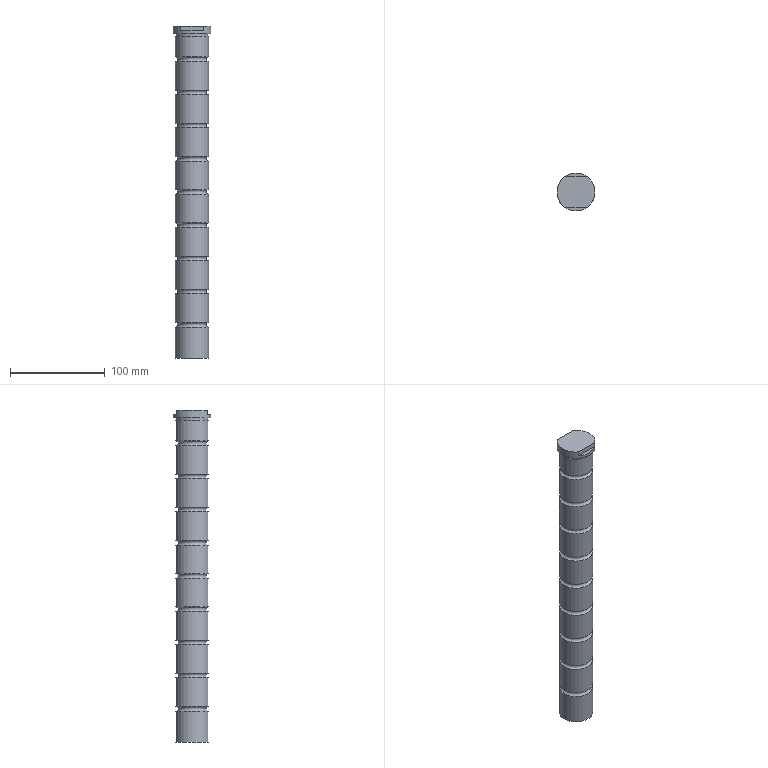Part | STEP file | 1_id442_xmt_txt | 1 solid | 33 faces | box 40 x 40 x 350 mm | volume 322067 mm3 | cylinder 14 | torus 9 | plane 8 | cone 2 | commonest cylinder face diameters 35 x10 13.6 x1 16 x1 33 x1 40 x1
STEP:
#1=CARTESIAN_POINT('',(144.5,302.,-131.5));
#2=VERTEX_POINT('',#1);
#3=CARTESIAN_POINT('',(162.,302.,-131.5));
#4=DIRECTION('',(0.,0.,-1.));
#5=DIRECTION('',(-1.,0.,0.));
#6=AXIS2_PLACEMENT_3D('',#3,#4,#5);
#7=CIRCLE('',#6,17.5);
#8=EDGE_CURVE('',#2,#2,#7,.T.);
#9=ORIENTED_EDGE('',*,*,#8,.F.);
#10=EDGE_LOOP('',(#9));
#11=FACE_BOUND('',#10,.T.);
#12=CARTESIAN_POINT('',(144.5,302.,-126.5));
#13=VERTEX_POINT('',#12);
#14=CARTESIAN_POINT('',(162.,302.,-126.5));
#15=DIRECTION('',(0.,0.,1.));
#16=DIRECTION('',(-1.,0.,0.));
#17=AXIS2_PLACEMENT_3D('',#14,#15,#16);
#18=CIRCLE('',#17,17.5);
#19=EDGE_CURVE('',#13,#13,#18,.T.);
#20=ORIENTED_EDGE('',*,*,#19,.F.);
#21=EDGE_LOOP('',(#20));
#22=FACE_BOUND('',#21,.T.);
#23=CARTESIAN_POINT('',(162.,302.,-129.));
#24=DIRECTION('',(0.,0.,-1.));
#25=DIRECTION('',(1.,0.,0.));
#26=AXIS2_PLACEMENT_3D('',#23,#24,#25);
#27=TOROIDAL_SURFACE('',#26,17.5,2.5);
#28=ADVANCED_FACE('',(#11,#22),#27,.F.);
#29=CARTESIAN_POINT('',(144.5,302.,-96.5));
#30=VERTEX_POINT('',#29);
#31=CARTESIAN_POINT('',(162.,302.,-96.5));
#32=DIRECTION('',(0.,0.,-1.));
#33=DIRECTION('',(-1.,0.,0.));
#34=AXIS2_PLACEMENT_3D('',#31,#32,#33);
#35=CIRCLE('',#34,17.5);
#36=EDGE_CURVE('',#30,#30,#35,.T.);
#37=ORIENTED_EDGE('',*,*,#36,.F.);
#38=EDGE_LOOP('',(#37));
#39=FACE_BOUND('',#38,.T.);
#40=CARTESIAN_POINT('',(144.5,302.,-91.5));
#41=VERTEX_POINT('',#40);
#42=CARTESIAN_POINT('',(162.,302.,-91.5));
#43=DIRECTION('',(0.,0.,1.));
#44=DIRECTION('',(-1.,0.,0.));
#45=AXIS2_PLACEMENT_3D('',#42,#43,#44);
#46=CIRCLE('',#45,17.5);
#47=EDGE_CURVE('',#41,#41,#46,.T.);
#48=ORIENTED_EDGE('',*,*,#47,.F.);
#49=EDGE_LOOP('',(#48));
#50=FACE_BOUND('',#49,.T.);
#51=CARTESIAN_POINT('',(162.,302.,-94.));
#52=DIRECTION('',(0.,0.,-1.));
#53=DIRECTION('',(1.,0.,0.));
#54=AXIS2_PLACEMENT_3D('',#51,#52,#53);
#55=TOROIDAL_SURFACE('',#54,17.5,2.5);
#56=ADVANCED_FACE('',(#39,#50),#55,.F.);
#57=CARTESIAN_POINT('',(144.5,302.,-61.5));
#58=VERTEX_POINT('',#57);
#59=CARTESIAN_POINT('',(162.,302.,-61.5));
#60=DIRECTION('',(0.,0.,-1.));
#61=DIRECTION('',(-1.,0.,0.));
#62=AXIS2_PLACEMENT_3D('',#59,#60,#61);
#63=CIRCLE('',#62,17.5);
#64=EDGE_CURVE('',#58,#58,#63,.T.);
#65=ORIENTED_EDGE('',*,*,#64,.F.);
#66=EDGE_LOOP('',(#65));
#67=FACE_BOUND('',#66,.T.);
#68=CARTESIAN_POINT('',(144.5,302.,-56.5));
#69=VERTEX_POINT('',#68);
#70=CARTESIAN_POINT('',(162.,302.,-56.5));
#71=DIRECTION('',(0.,0.,1.));
#72=DIRECTION('',(-1.,0.,0.));
#73=AXIS2_PLACEMENT_3D('',#70,#71,#72);
#74=CIRCLE('',#73,17.5);
#75=EDGE_CURVE('',#69,#69,#74,.T.);
#76=ORIENTED_EDGE('',*,*,#75,.F.);
#77=EDGE_LOOP('',(#76));
#78=FACE_BOUND('',#77,.T.);
#79=CARTESIAN_POINT('',(162.,302.,-59.));
#80=DIRECTION('',(0.,0.,-1.));
#81=DIRECTION('',(1.,0.,0.));
#82=AXIS2_PLACEMENT_3D('',#79,#80,#81);
#83=TOROIDAL_SURFACE('',#82,17.5,2.5);
#84=ADVANCED_FACE('',(#67,#78),#83,.F.);
#85=CARTESIAN_POINT('',(144.5,302.,-26.5));
#86=VERTEX_POINT('',#85);
#87=CARTESIAN_POINT('',(162.,302.,-26.5));
#88=DIRECTION('',(0.,0.,-1.));
#89=DIRECTION('',(-1.,0.,0.));
#90=AXIS2_PLACEMENT_3D('',#87,#88,#89);
#91=CIRCLE('',#90,17.5);
#92=EDGE_CURVE('',#86,#86,#91,.T.);
#93=ORIENTED_EDGE('',*,*,#92,.F.);
#94=EDGE_LOOP('',(#93));
#95=FACE_BOUND('',#94,.T.);
#96=CARTESIAN_POINT('',(144.5,302.,-21.5));
#97=VERTEX_POINT('',#96);
#98=CARTESIAN_POINT('',(162.,302.,-21.5));
#99=DIRECTION('',(0.,0.,1.));
#100=DIRECTION('',(-1.,0.,0.));
#101=AXIS2_PLACEMENT_3D('',#98,#99,#100);
#102=CIRCLE('',#101,17.5);
#103=EDGE_CURVE('',#97,#97,#102,.T.);
#104=ORIENTED_EDGE('',*,*,#103,.F.);
#105=EDGE_LOOP('',(#104));
#106=FACE_BOUND('',#105,.T.);
#107=CARTESIAN_POINT('',(162.,302.,-24.));
#108=DIRECTION('',(0.,0.,-1.));
#109=DIRECTION('',(1.,0.,0.));
#110=AXIS2_PLACEMENT_3D('',#107,#108,#109);
#111=TOROIDAL_SURFACE('',#110,17.5,2.5);
#112=ADVANCED_FACE('',(#95,#106),#111,.F.);
#113=CARTESIAN_POINT('',(144.5,302.,8.5));
#114=VERTEX_POINT('',#113);
#115=CARTESIAN_POINT('',(162.,302.,8.5));
#116=DIRECTION('',(0.,0.,-1.));
#117=DIRECTION('',(-1.,0.,0.));
#118=AXIS2_PLACEMENT_3D('',#115,#116,#117);
#119=CIRCLE('',#118,17.5);
#120=EDGE_CURVE('',#114,#114,#119,.T.);
#121=ORIENTED_EDGE('',*,*,#120,.F.);
#122=EDGE_LOOP('',(#121));
#123=FACE_BOUND('',#122,.T.);
#124=CARTESIAN_POINT('',(144.5,302.,13.5));
#125=VERTEX_POINT('',#124);
#126=CARTESIAN_POINT('',(162.,302.,13.5));
#127=DIRECTION('',(0.,0.,1.));
#128=DIRECTION('',(-1.,0.,0.));
#129=AXIS2_PLACEMENT_3D('',#126,#127,#128);
#130=CIRCLE('',#129,17.5);
#131=EDGE_CURVE('',#125,#125,#130,.T.);
#132=ORIENTED_EDGE('',*,*,#131,.F.);
#133=EDGE_LOOP('',(#132));
#134=FACE_BOUND('',#133,.T.);
#135=CARTESIAN_POINT('',(162.,302.,11.));
#136=DIRECTION('',(0.,0.,-1.));
#137=DIRECTION('',(1.,0.,0.));
#138=AXIS2_PLACEMENT_3D('',#135,#136,#137);
#139=TOROIDAL_SURFACE('',#138,17.5,2.5);
#140=ADVANCED_FACE('',(#123,#134),#139,.F.);
#141=CARTESIAN_POINT('',(144.5,302.,43.5));
#142=VERTEX_POINT('',#141);
#143=CARTESIAN_POINT('',(162.,302.,43.5));
#144=DIRECTION('',(0.,0.,-1.));
#145=DIRECTION('',(-1.,0.,0.));
#146=AXIS2_PLACEMENT_3D('',#143,#144,#145);
#147=CIRCLE('',#146,17.5);
#148=EDGE_CURVE('',#142,#142,#147,.T.);
#149=ORIENTED_EDGE('',*,*,#148,.F.);
#150=EDGE_LOOP('',(#149));
#151=FACE_BOUND('',#150,.T.);
#152=CARTESIAN_POINT('',(144.5,302.,48.5));
#153=VERTEX_POINT('',#152);
#154=CARTESIAN_POINT('',(162.,302.,48.5));
#155=DIRECTION('',(0.,0.,1.));
#156=DIRECTION('',(-1.,0.,0.));
#157=AXIS2_PLACEMENT_3D('',#154,#155,#156);
#158=CIRCLE('',#157,17.5);
#159=EDGE_CURVE('',#153,#153,#158,.T.);
#160=ORIENTED_EDGE('',*,*,#159,.F.);
#161=EDGE_LOOP('',(#160));
#162=FACE_BOUND('',#161,.T.);
#163=CARTESIAN_POINT('',(162.,302.,46.));
#164=DIRECTION('',(0.,0.,-1.));
#165=DIRECTION('',(1.,0.,0.));
#166=AXIS2_PLACEMENT_3D('',#163,#164,#165);
#167=TOROIDAL_SURFACE('',#166,17.5,2.5);
#168=ADVANCED_FACE('',(#151,#162),#167,.F.);
#169=CARTESIAN_POINT('',(144.5,302.,78.5));
#170=VERTEX_POINT('',#169);
#171=CARTESIAN_POINT('',(162.,302.,78.5));
#172=DIRECTION('',(0.,0.,-1.));
#173=DIRECTION('',(-1.,0.,0.));
#174=AXIS2_PLACEMENT_3D('',#171,#172,#173);
#175=CIRCLE('',#174,17.5);
#176=EDGE_CURVE('',#170,#170,#175,.T.);
#177=ORIENTED_EDGE('',*,*,#176,.F.);
#178=EDGE_LOOP('',(#177));
#179=FACE_BOUND('',#178,.T.);
#180=CARTESIAN_POINT('',(144.5,302.,83.5));
#181=VERTEX_POINT('',#180);
#182=CARTESIAN_POINT('',(162.,302.,83.5));
#183=DIRECTION('',(0.,0.,1.));
#184=DIRECTION('',(-1.,0.,0.));
#185=AXIS2_PLACEMENT_3D('',#182,#183,#184);
#186=CIRCLE('',#185,17.5);
#187=EDGE_CURVE('',#181,#181,#186,.T.);
#188=ORIENTED_EDGE('',*,*,#187,.F.);
#189=EDGE_LOOP('',(#188));
#190=FACE_BOUND('',#189,.T.);
#191=CARTESIAN_POINT('',(162.,302.,81.));
#192=DIRECTION('',(0.,0.,-1.));
#193=DIRECTION('',(1.,0.,0.));
#194=AXIS2_PLACEMENT_3D('',#191,#192,#193);
#195=TOROIDAL_SURFACE('',#194,17.5,2.5);
#196=ADVANCED_FACE('',(#179,#190),#195,.F.);
#197=CARTESIAN_POINT('',(144.5,302.,113.5));
#198=VERTEX_POINT('',#197);
#199=CARTESIAN_POINT('',(162.,302.,113.5));
#200=DIRECTION('',(0.,0.,-1.));
#201=DIRECTION('',(-1.,0.,0.));
#202=AXIS2_PLACEMENT_3D('',#199,#200,#201);
#203=CIRCLE('',#202,17.5);
#204=EDGE_CURVE('',#198,#198,#203,.T.);
#205=ORIENTED_EDGE('',*,*,#204,.F.);
#206=EDGE_LOOP('',(#205));
#207=FACE_BOUND('',#206,.T.);
#208=CARTESIAN_POINT('',(144.5,302.,118.5));
#209=VERTEX_POINT('',#208);
#210=CARTESIAN_POINT('',(162.,302.,118.5));
#211=DIRECTION('',(0.,0.,1.));
#212=DIRECTION('',(-1.,0.,0.));
#213=AXIS2_PLACEMENT_3D('',#210,#211,#212);
#214=CIRCLE('',#213,17.5);
#215=EDGE_CURVE('',#209,#209,#214,.T.);
#216=ORIENTED_EDGE('',*,*,#215,.F.);
#217=EDGE_LOOP('',(#216));
#218=FACE_BOUND('',#217,.T.);
#219=CARTESIAN_POINT('',(162.,302.,116.));
#220=DIRECTION('',(0.,0.,-1.));
#221=DIRECTION('',(1.,0.,0.));
#222=AXIS2_PLACEMENT_3D('',#219,#220,#221);
#223=TOROIDAL_SURFACE('',#222,17.5,2.5);
#224=ADVANCED_FACE('',(#207,#218),#223,.F.);
#225=CARTESIAN_POINT('',(144.5,302.,148.5));
#226=VERTEX_POINT('',#225);
#227=CARTESIAN_POINT('',(162.,302.,148.5));
#228=DIRECTION('',(0.,0.,-1.));
#229=DIRECTION('',(-1.,0.,0.));
#230=AXIS2_PLACEMENT_3D('',#227,#228,#229);
#231=CIRCLE('',#230,17.5);
#232=EDGE_CURVE('',#226,#226,#231,.T.);
#233=ORIENTED_EDGE('',*,*,#232,.F.);
#234=EDGE_LOOP('',(#233));
#235=FACE_BOUND('',#234,.T.);
#236=CARTESIAN_POINT('',(144.5,302.,153.5));
#237=VERTEX_POINT('',#236);
#238=CARTESIAN_POINT('',(162.,302.,153.5));
#239=DIRECTION('',(0.,0.,1.));
#240=DIRECTION('',(-1.,0.,0.));
#241=AXIS2_PLACEMENT_3D('',#238,#239,#240);
#242=CIRCLE('',#241,17.5);
#243=EDGE_CURVE('',#237,#237,#242,.T.);
#244=ORIENTED_EDGE('',*,*,#243,.F.);
#245=EDGE_LOOP('',(#244));
#246=FACE_BOUND('',#245,.T.);
#247=CARTESIAN_POINT('',(162.,302.,151.));
#248=DIRECTION('',(0.,0.,-1.));
#249=DIRECTION('',(1.,0.,0.));
#250=AXIS2_PLACEMENT_3D('',#247,#248,#249);
#251=TOROIDAL_SURFACE('',#250,17.5,2.5);
#252=ADVANCED_FACE('',(#235,#246),#251,.F.);
#253=ORIENTED_EDGE('',*,*,#8,.T.);
#254=EDGE_LOOP('',(#253));
#255=FACE_BOUND('',#254,.T.);
#256=CARTESIAN_POINT('',(144.5,302.,-164.));
#257=VERTEX_POINT('',#256);
#258=CARTESIAN_POINT('',(162.,302.,-164.));
#259=DIRECTION('',(0.,0.,-1.));
#260=DIRECTION('',(-1.,0.,0.));
#261=AXIS2_PLACEMENT_3D('',#258,#259,#260);
#262=CIRCLE('',#261,17.5);
#263=EDGE_CURVE('',#257,#257,#262,.T.);
#264=ORIENTED_EDGE('',*,*,#263,.F.);
#265=EDGE_LOOP('',(#264));
#266=FACE_BOUND('',#265,.T.);
#267=CARTESIAN_POINT('',(162.,302.,7.));
#268=DIRECTION('',(0.,0.,-1.));
#269=DIRECTION('',(1.,0.,0.));
#270=AXIS2_PLACEMENT_3D('',#267,#268,#269);
#271=CYLINDRICAL_SURFACE('',#270,17.5);
#272=ADVANCED_FACE('',(#255,#266),#271,.T.);
#273=CARTESIAN_POINT('',(178.5,302.,175.));
#274=VERTEX_POINT('',#273);
#275=CARTESIAN_POINT('',(162.,302.,175.));
#276=DIRECTION('',(0.,0.,-1.));
#277=DIRECTION('',(1.,0.,0.));
#278=AXIS2_PLACEMENT_3D('',#275,#276,#277);
#279=CIRCLE('',#278,16.5);
#280=EDGE_CURVE('',#274,#274,#279,.T.);
#281=ORIENTED_EDGE('',*,*,#280,.F.);
#282=EDGE_LOOP('',(#281));
#283=FACE_BOUND('',#282,.T.);
#284=CARTESIAN_POINT('',(178.5,302.,178.));
#285=VERTEX_POINT('',#284);
#286=CARTESIAN_POINT('',(162.,302.,178.));
#287=DIRECTION('',(0.,0.,1.));
#288=DIRECTION('',(1.,0.,0.));
#289=AXIS2_PLACEMENT_3D('',#286,#287,#288);
#290=CIRCLE('',#289,16.5);
#291=EDGE_CURVE('',#285,#285,#290,.T.);
#292=ORIENTED_EDGE('',*,*,#291,.F.);
#293=EDGE_LOOP('',(#292));
#294=FACE_BOUND('',#293,.T.);
#295=CARTESIAN_POINT('',(162.,302.,176.5));
#296=DIRECTION('',(0.,0.,-1.));
#297=DIRECTION('',(-1.,0.,0.));
#298=AXIS2_PLACEMENT_3D('',#295,#296,#297);
#299=CYLINDRICAL_SURFACE('',#298,16.5);
#300=ADVANCED_FACE('',(#283,#294),#299,.T.);
#301=CARTESIAN_POINT('',(174.,286.,186.));
#302=VERTEX_POINT('',#301);
#303=CARTESIAN_POINT('',(174.,318.,186.));
#304=VERTEX_POINT('',#303);
#305=CARTESIAN_POINT('',(162.,302.,186.));
#306=DIRECTION('',(0.,0.,1.));
#307=DIRECTION('',(-1.,0.,0.));
#308=AXIS2_PLACEMENT_3D('',#305,#306,#307);
#309=CIRCLE('',#308,20.);
#310=EDGE_CURVE('',#302,#304,#309,.T.);
#311=ORIENTED_EDGE('',*,*,#310,.F.);
#312=CARTESIAN_POINT('',(174.,286.,181.));
#313=VERTEX_POINT('',#312);
#314=CARTESIAN_POINT('',(174.,286.,183.5));
#315=DIRECTION('',(0.,0.,-1.));
#316=VECTOR('',#315,1.);
#317=LINE('',#314,#316);
#318=EDGE_CURVE('',#302,#313,#317,.T.);
#319=ORIENTED_EDGE('',*,*,#318,.T.);
#320=CARTESIAN_POINT('',(150.,286.,181.));
#321=VERTEX_POINT('',#320);
#322=CARTESIAN_POINT('',(162.,302.,181.));
#323=DIRECTION('',(0.,0.,-1.));
#324=DIRECTION('',(-1.,0.,0.));
#325=AXIS2_PLACEMENT_3D('',#322,#323,#324);
#326=CIRCLE('',#325,20.);
#327=EDGE_CURVE('',#313,#321,#326,.T.);
#328=ORIENTED_EDGE('',*,*,#327,.T.);
#329=CARTESIAN_POINT('',(150.,286.,186.));
#330=VERTEX_POINT('',#329);
#331=CARTESIAN_POINT('',(150.,286.,183.5));
#332=DIRECTION('',(0.,0.,1.));
#333=VECTOR('',#332,1.);
#334=LINE('',#331,#333);
#335=EDGE_CURVE('',#321,#330,#334,.T.);
#336=ORIENTED_EDGE('',*,*,#335,.T.);
#337=CARTESIAN_POINT('',(150.,318.,186.));
#338=VERTEX_POINT('',#337);
#339=CARTESIAN_POINT('',(162.,302.,186.));
#340=DIRECTION('',(0.,0.,1.));
#341=DIRECTION('',(-1.,0.,0.));
#342=AXIS2_PLACEMENT_3D('',#339,#340,#341);
#343=CIRCLE('',#342,20.);
#344=EDGE_CURVE('',#338,#330,#343,.T.);
#345=ORIENTED_EDGE('',*,*,#344,.F.);
#346=CARTESIAN_POINT('',(150.,318.,181.));
#347=VERTEX_POINT('',#346);
#348=CARTESIAN_POINT('',(150.,318.,183.5));
#349=DIRECTION('',(0.,0.,-1.));
#350=VECTOR('',#349,1.);
#351=LINE('',#348,#350);
#352=EDGE_CURVE('',#338,#347,#351,.T.);
#353=ORIENTED_EDGE('',*,*,#352,.T.);
#354=CARTESIAN_POINT('',(174.,318.,181.));
#355=VERTEX_POINT('',#354);
#356=CARTESIAN_POINT('',(162.,302.,181.));
#357=DIRECTION('',(0.,0.,-1.));
#358=DIRECTION('',(-1.,0.,0.));
#359=AXIS2_PLACEMENT_3D('',#356,#357,#358);
#360=CIRCLE('',#359,20.);
#361=EDGE_CURVE('',#347,#355,#360,.T.);
#362=ORIENTED_EDGE('',*,*,#361,.T.);
#363=CARTESIAN_POINT('',(174.,318.,183.5));
#364=DIRECTION('',(0.,0.,1.));
#365=VECTOR('',#364,1.);
#366=LINE('',#363,#365);
#367=EDGE_CURVE('',#355,#304,#366,.T.);
#368=ORIENTED_EDGE('',*,*,#367,.T.);
#369=EDGE_LOOP('',(#311,#319,#328,#336,#345,#353,#362,#368));
#370=FACE_BOUND('',#369,.T.);
#371=CARTESIAN_POINT('',(142.,302.,178.));
#372=VERTEX_POINT('',#371);
#373=CARTESIAN_POINT('',(162.,302.,178.));
#374=DIRECTION('',(0.,0.,-1.));
#375=DIRECTION('',(-1.,0.,0.));
#376=AXIS2_PLACEMENT_3D('',#373,#374,#375);
#377=CIRCLE('',#376,20.);
#378=EDGE_CURVE('',#372,#372,#377,.T.);
#379=ORIENTED_EDGE('',*,*,#378,.F.);
#380=EDGE_LOOP('',(#379));
#381=FACE_BOUND('',#380,.T.);
#382=CARTESIAN_POINT('',(162.,302.,182.));
#383=DIRECTION('',(0.,0.,-1.));
#384=DIRECTION('',(1.,0.,0.));
#385=AXIS2_PLACEMENT_3D('',#382,#383,#384);
#386=CYLINDRICAL_SURFACE('',#385,20.);
#387=ADVANCED_FACE('',(#370,#381),#386,.T.);
#388=ORIENTED_EDGE('',*,*,#36,.T.);
#389=EDGE_LOOP('',(#388));
#390=FACE_BOUND('',#389,.T.);
#391=ORIENTED_EDGE('',*,*,#19,.T.);
#392=EDGE_LOOP('',(#391));
#393=FACE_BOUND('',#392,.T.);
#394=CARTESIAN_POINT('',(162.,302.,7.));
#395=DIRECTION('',(0.,0.,-1.));
#396=DIRECTION('',(1.,0.,0.));
#397=AXIS2_PLACEMENT_3D('',#394,#395,#396);
#398=CYLINDRICAL_SURFACE('',#397,17.5);
#399=ADVANCED_FACE('',(#390,#393),#398,.T.);
#400=ORIENTED_EDGE('',*,*,#64,.T.);
#401=EDGE_LOOP('',(#400));
#402=FACE_BOUND('',#401,.T.);
#403=ORIENTED_EDGE('',*,*,#47,.T.);
#404=EDGE_LOOP('',(#403));
#405=FACE_BOUND('',#404,.T.);
#406=CARTESIAN_POINT('',(162.,302.,7.));
#407=DIRECTION('',(0.,0.,-1.));
#408=DIRECTION('',(1.,0.,0.));
#409=AXIS2_PLACEMENT_3D('',#406,#407,#408);
#410=CYLINDRICAL_SURFACE('',#409,17.5);
#411=ADVANCED_FACE('',(#402,#405),#410,.T.);
#412=ORIENTED_EDGE('',*,*,#92,.T.);
#413=EDGE_LOOP('',(#412));
#414=FACE_BOUND('',#413,.T.);
#415=ORIENTED_EDGE('',*,*,#75,.T.);
#416=EDGE_LOOP('',(#415));
#417=FACE_BOUND('',#416,.T.);
#418=CARTESIAN_POINT('',(162.,302.,7.));
#419=DIRECTION('',(0.,0.,-1.));
#420=DIRECTION('',(1.,0.,0.));
#421=AXIS2_PLACEMENT_3D('',#418,#419,#420);
#422=CYLINDRICAL_SURFACE('',#421,17.5);
#423=ADVANCED_FACE('',(#414,#417),#422,.T.);
#424=ORIENTED_EDGE('',*,*,#120,.T.);
#425=EDGE_LOOP('',(#424));
#426=FACE_BOUND('',#425,.T.);
#427=ORIENTED_EDGE('',*,*,#103,.T.);
#428=EDGE_LOOP('',(#427));
#429=FACE_BOUND('',#428,.T.);
#430=CARTESIAN_POINT('',(162.,302.,7.));
#431=DIRECTION('',(0.,0.,-1.));
#432=DIRECTION('',(1.,0.,0.));
#433=AXIS2_PLACEMENT_3D('',#430,#431,#432);
#434=CYLINDRICAL_SURFACE('',#433,17.5);
#435=ADVANCED_FACE('',(#426,#429),#434,.T.);
#436=ORIENTED_EDGE('',*,*,#148,.T.);
#437=EDGE_LOOP('',(#436));
#438=FACE_BOUND('',#437,.T.);
#439=ORIENTED_EDGE('',*,*,#131,.T.);
#440=EDGE_LOOP('',(#439));
#441=FACE_BOUND('',#440,.T.);
#442=CARTESIAN_POINT('',(162.,302.,7.));
#443=DIRECTION('',(0.,0.,-1.));
#444=DIRECTION('',(1.,0.,0.));
#445=AXIS2_PLACEMENT_3D('',#442,#443,#444);
#446=CYLINDRICAL_SURFACE('',#445,17.5);
#447=ADVANCED_FACE('',(#438,#441),#446,.T.);
#448=ORIENTED_EDGE('',*,*,#176,.T.);
#449=EDGE_LOOP('',(#448));
#450=FACE_BOUND('',#449,.T.);
#451=ORIENTED_EDGE('',*,*,#159,.T.);
#452=EDGE_LOOP('',(#451));
#453=FACE_BOUND('',#452,.T.);
#454=CARTESIAN_POINT('',(162.,302.,7.));
#455=DIRECTION('',(0.,0.,-1.));
#456=DIRECTION('',(1.,0.,0.));
#457=AXIS2_PLACEMENT_3D('',#454,#455,#456);
#458=CYLINDRICAL_SURFACE('',#457,17.5);
#459=ADVANCED_FACE('',(#450,#453),#458,.T.);
#460=ORIENTED_EDGE('',*,*,#204,.T.);
#461=EDGE_LOOP('',(#460));
#462=FACE_BOUND('',#461,.T.);
#463=ORIENTED_EDGE('',*,*,#187,.T.);
#464=EDGE_LOOP('',(#463));
#465=FACE_BOUND('',#464,.T.);
#466=CARTESIAN_POINT('',(162.,302.,7.));
#467=DIRECTION('',(0.,0.,-1.));
#468=DIRECTION('',(1.,0.,0.));
#469=AXIS2_PLACEMENT_3D('',#466,#467,#468);
#470=CYLINDRICAL_SURFACE('',#469,17.5);
#471=ADVANCED_FACE('',(#462,#465),#470,.T.);
#472=ORIENTED_EDGE('',*,*,#232,.T.);
#473=EDGE_LOOP('',(#472));
#474=FACE_BOUND('',#473,.T.);
#475=ORIENTED_EDGE('',*,*,#215,.T.);
#476=EDGE_LOOP('',(#475));
#477=FACE_BOUND('',#476,.T.);
#478=CARTESIAN_POINT('',(162.,302.,7.));
#479=DIRECTION('',(0.,0.,-1.));
#480=DIRECTION('',(1.,0.,0.));
#481=AXIS2_PLACEMENT_3D('',#478,#479,#480);
#482=CYLINDRICAL_SURFACE('',#481,17.5);
#483=ADVANCED_FACE('',(#474,#477),#482,.T.);
#484=CARTESIAN_POINT('',(144.5,302.,175.));
#485=VERTEX_POINT('',#484);
#486=CARTESIAN_POINT('',(162.,302.,175.));
#487=DIRECTION('',(0.,0.,-1.));
#488=DIRECTION('',(-1.,0.,0.));
#489=AXIS2_PLACEMENT_3D('',#486,#487,#488);
#490=CIRCLE('',#489,17.5);
#491=EDGE_CURVE('',#485,#485,#490,.T.);
#492=ORIENTED_EDGE('',*,*,#491,.T.);
#493=EDGE_LOOP('',(#492));
#494=FACE_BOUND('',#493,.T.);
#495=ORIENTED_EDGE('',*,*,#243,.T.);
#496=EDGE_LOOP('',(#495));
#497=FACE_BOUND('',#496,.T.);
#498=CARTESIAN_POINT('',(162.,302.,7.));
#499=DIRECTION('',(0.,0.,-1.));
#500=DIRECTION('',(1.,0.,0.));
#501=AXIS2_PLACEMENT_3D('',#498,#499,#500);
#502=CYLINDRICAL_SURFACE('',#501,17.5);
#503=ADVANCED_FACE('',(#494,#497),#502,.T.);
#504=CARTESIAN_POINT('',(170.,302.,-132.));
#505=VERTEX_POINT('',#504);
#506=CARTESIAN_POINT('',(162.,302.,-132.));
#507=DIRECTION('',(0.,0.,1.));
#508=DIRECTION('',(1.,0.,0.));
#509=AXIS2_PLACEMENT_3D('',#506,#507,#508);
#510=CIRCLE('',#509,8.);
#511=EDGE_CURVE('',#505,#505,#510,.T.);
#512=ORIENTED_EDGE('',*,*,#511,.T.);
#513=EDGE_LOOP('',(#512));
#514=FACE_BOUND('',#513,.T.);
#515=CARTESIAN_POINT('',(170.,302.,-164.));
#516=VERTEX_POINT('',#515);
#517=CARTESIAN_POINT('',(162.,302.,-164.));
#518=DIRECTION('',(0.,0.,1.));
#519=DIRECTION('',(1.,0.,0.));
#520=AXIS2_PLACEMENT_3D('',#517,#518,#519);
#521=CIRCLE('',#520,8.);
#522=EDGE_CURVE('',#516,#516,#521,.T.);
#523=ORIENTED_EDGE('',*,*,#522,.F.);
#524=EDGE_LOOP('',(#523));
#525=FACE_BOUND('',#524,.T.);
#526=CARTESIAN_POINT('',(162.,302.,-148.));
#527=DIRECTION('',(0.,0.,1.));
#528=DIRECTION('',(-1.,0.,0.));
#529=AXIS2_PLACEMENT_3D('',#526,#527,#528);
#530=CYLINDRICAL_SURFACE('',#529,8.);
#531=ADVANCED_FACE('',(#514,#525),#530,.F.);
#532=CARTESIAN_POINT('',(168.8,302.,-131.5));
#533=VERTEX_POINT('',#532);
#534=CARTESIAN_POINT('',(162.,302.,-131.5));
#535=DIRECTION('',(0.,0.,1.));
#536=DIRECTION('',(1.,0.,0.));
#537=AXIS2_PLACEMENT_3D('',#534,#535,#536);
#538=CIRCLE('',#537,6.8);
#539=EDGE_CURVE('',#533,#533,#538,.T.);
#540=ORIENTED_EDGE('',*,*,#539,.T.);
#541=EDGE_LOOP('',(#540));
#542=FACE_BOUND('',#541,.T.);
#543=ORIENTED_EDGE('',*,*,#511,.F.);
#544=EDGE_LOOP('',(#543));
#545=FACE_BOUND('',#544,.T.);
#546=CARTESIAN_POINT('',(162.,302.,-131.75));
#547=DIRECTION('',(0.,0.,-1.));
#548=DIRECTION('',(-1.,0.,0.));
#549=AXIS2_PLACEMENT_3D('',#546,#547,#548);
#550=CONICAL_SURFACE('',#549,7.4,67.38);
#551=ADVANCED_FACE('',(#542,#545),#550,.F.);
#552=CARTESIAN_POINT('',(168.8,302.,-130.));
#553=VERTEX_POINT('',#552);
#554=CARTESIAN_POINT('',(162.,302.,-130.));
#555=DIRECTION('',(0.,0.,1.));
#556=DIRECTION('',(1.,0.,0.));
#557=AXIS2_PLACEMENT_3D('',#554,#555,#556);
#558=CIRCLE('',#557,6.8);
#559=EDGE_CURVE('',#553,#553,#558,.T.);
#560=ORIENTED_EDGE('',*,*,#559,.T.);
#561=EDGE_LOOP('',(#560));
#562=FACE_BOUND('',#561,.T.);
#563=ORIENTED_EDGE('',*,*,#539,.F.);
#564=EDGE_LOOP('',(#563));
#565=FACE_BOUND('',#564,.T.);
#566=CARTESIAN_POINT('',(162.,302.,-130.75));
#567=DIRECTION('',(0.,0.,1.));
#568=DIRECTION('',(-1.,0.,0.));
#569=AXIS2_PLACEMENT_3D('',#566,#567,#568);
#570=CYLINDRICAL_SURFACE('',#569,6.8);
#571=ADVANCED_FACE('',(#562,#565),#570,.F.);
#572=ORIENTED_EDGE('',*,*,#559,.F.);
#573=EDGE_LOOP('',(#572));
#574=FACE_BOUND('',#573,.T.);
#575=CARTESIAN_POINT('',(162.,302.,-126.074));
#576=VERTEX_POINT('',#575);
#577=VERTEX_LOOP('',#576);
#578=FACE_BOUND('',#577,.T.);
#579=CARTESIAN_POINT('',(162.,302.,-128.037));
#580=DIRECTION('',(0.,0.,-1.));
#581=DIRECTION('',(-1.,0.,0.));
#582=AXIS2_PLACEMENT_3D('',#579,#580,#581);
#583=CONICAL_SURFACE('',#582,3.4,60.);
#584=ADVANCED_FACE('',(#574,#578),#583,.F.);
#585=ORIENTED_EDGE('',*,*,#367,.F.);
#586=CARTESIAN_POINT('',(162.,318.,181.));
#587=DIRECTION('',(-1.,0.,0.));
#588=VECTOR('',#587,1.);
#589=LINE('',#586,#588);
#590=EDGE_CURVE('',#355,#347,#589,.T.);
#591=ORIENTED_EDGE('',*,*,#590,.T.);
#592=ORIENTED_EDGE('',*,*,#352,.F.);
#593=CARTESIAN_POINT('',(162.,318.,186.));
#594=DIRECTION('',(-1.,0.,0.));
#595=VECTOR('',#594,1.);
#596=LINE('',#593,#595);
#597=EDGE_CURVE('',#304,#338,#596,.T.);
#598=ORIENTED_EDGE('',*,*,#597,.F.);
#599=EDGE_LOOP('',(#585,#591,#592,#598));
#600=FACE_OUTER_BOUND('',#599,.T.);
#601=CARTESIAN_POINT('',(162.,318.,183.5));
#602=DIRECTION('',(0.,1.,0.));
#603=DIRECTION('',(-1.,0.,0.));
#604=AXIS2_PLACEMENT_3D('',#601,#602,#603);
#605=PLANE('',#604);
#606=ADVANCED_FACE('',(#600),#605,.T.);
#607=ORIENTED_EDGE('',*,*,#361,.F.);
#608=ORIENTED_EDGE('',*,*,#590,.F.);
#609=EDGE_LOOP('',(#607,#608));
#610=FACE_OUTER_BOUND('',#609,.T.);
#611=CARTESIAN_POINT('',(162.,320.,181.));
#612=DIRECTION('',(0.,0.,1.));
#613=DIRECTION('',(-1.,0.,0.));
#614=AXIS2_PLACEMENT_3D('',#611,#612,#613);
#615=PLANE('',#614);
#616=ADVANCED_FACE('',(#610),#615,.T.);
#617=ORIENTED_EDGE('',*,*,#597,.T.);
#618=ORIENTED_EDGE('',*,*,#344,.T.);
#619=CARTESIAN_POINT('',(162.,286.,186.));
#620=DIRECTION('',(1.,0.,0.));
#621=VECTOR('',#620,1.);
#622=LINE('',#619,#621);
#623=EDGE_CURVE('',#330,#302,#622,.T.);
#624=ORIENTED_EDGE('',*,*,#623,.T.);
#625=ORIENTED_EDGE('',*,*,#310,.T.);
#626=EDGE_LOOP('',(#617,#618,#624,#625));
#627=FACE_OUTER_BOUND('',#626,.T.);
#628=CARTESIAN_POINT('',(162.,302.,186.));
#629=DIRECTION('',(0.,0.,1.));
#630=DIRECTION('',(-1.,0.,0.));
#631=AXIS2_PLACEMENT_3D('',#628,#629,#630);
#632=PLANE('',#631);
#633=ADVANCED_FACE('',(#627),#632,.T.);
#634=ORIENTED_EDGE('',*,*,#318,.F.);
#635=ORIENTED_EDGE('',*,*,#623,.F.);
#636=ORIENTED_EDGE('',*,*,#335,.F.);
#637=CARTESIAN_POINT('',(162.,286.,181.));
#638=DIRECTION('',(-1.,0.,0.));
#639=VECTOR('',#638,1.);
#640=LINE('',#637,#639);
#641=EDGE_CURVE('',#313,#321,#640,.T.);
#642=ORIENTED_EDGE('',*,*,#641,.F.);
#643=EDGE_LOOP('',(#634,#635,#636,#642));
#644=FACE_OUTER_BOUND('',#643,.T.);
#645=CARTESIAN_POINT('',(162.,286.,183.5));
#646=DIRECTION('',(0.,-1.,0.));
#647=DIRECTION('',(1.,0.,0.));
#648=AXIS2_PLACEMENT_3D('',#645,#646,#647);
#649=PLANE('',#648);
#650=ADVANCED_FACE('',(#644),#649,.T.);
#651=ORIENTED_EDGE('',*,*,#327,.F.);
#652=ORIENTED_EDGE('',*,*,#641,.T.);
#653=EDGE_LOOP('',(#651,#652));
#654=FACE_OUTER_BOUND('',#653,.T.);
#655=CARTESIAN_POINT('',(162.,284.,181.));
#656=DIRECTION('',(0.,0.,1.));
#657=DIRECTION('',(-1.,0.,0.));
#658=AXIS2_PLACEMENT_3D('',#655,#656,#657);
#659=PLANE('',#658);
#660=ADVANCED_FACE('',(#654),#659,.T.);
#661=ORIENTED_EDGE('',*,*,#280,.T.);
#662=EDGE_LOOP('',(#661));
#663=FACE_BOUND('',#662,.T.);
#664=ORIENTED_EDGE('',*,*,#491,.F.);
#665=EDGE_LOOP('',(#664));
#666=FACE_BOUND('',#665,.T.);
#667=CARTESIAN_POINT('',(179.,302.,175.));
#668=DIRECTION('',(0.,0.,-1.));
#669=DIRECTION('',(-1.,0.,0.));
#670=AXIS2_PLACEMENT_3D('',#667,#668,#669);
#671=PLANE('',#670);
#672=ADVANCED_FACE('',(#663,#666),#671,.F.);
#673=ORIENTED_EDGE('',*,*,#522,.T.);
#674=EDGE_LOOP('',(#673));
#675=FACE_BOUND('',#674,.T.);
#676=ORIENTED_EDGE('',*,*,#263,.T.);
#677=EDGE_LOOP('',(#676));
#678=FACE_BOUND('',#677,.T.);
#679=CARTESIAN_POINT('',(162.,302.,-164.));
#680=DIRECTION('',(0.,0.,-1.));
#681=DIRECTION('',(1.,0.,0.));
#682=AXIS2_PLACEMENT_3D('',#679,#680,#681);
#683=PLANE('',#682);
#684=ADVANCED_FACE('',(#675,#678),#683,.T.);
#685=ORIENTED_EDGE('',*,*,#291,.T.);
#686=EDGE_LOOP('',(#685));
#687=FACE_BOUND('',#686,.T.);
#688=ORIENTED_EDGE('',*,*,#378,.T.);
#689=EDGE_LOOP('',(#688));
#690=FACE_BOUND('',#689,.T.);
#691=CARTESIAN_POINT('',(162.,302.,178.));
#692=DIRECTION('',(0.,0.,-1.));
#693=DIRECTION('',(1.,0.,0.));
#694=AXIS2_PLACEMENT_3D('',#691,#692,#693);
#695=PLANE('',#694);
#696=ADVANCED_FACE('',(#687,#690),#695,.T.);
#697=CLOSED_SHELL('',(#28,#56,#84,#112,#140,#168,#196,#224,#252,#272,#300,#387,#399,#411,#423,#435,#447,#459,#471,#483,#503,#531,#551,#571,#584,#606,#616,#633,#650,#660,#672,#684,#696));
#698=MANIFOLD_SOLID_BREP('',#697);
#699=(LENGTH_UNIT()NAMED_UNIT(*)SI_UNIT(.MILLI.,.METRE.));
#700=UNCERTAINTY_MEASURE_WITH_UNIT(LENGTH_MEASURE(0.00002),#699,'','');
#701=(NAMED_UNIT(*)PLANE_ANGLE_UNIT()SI_UNIT($,.RADIAN.));
#702=PLANE_ANGLE_MEASURE_WITH_UNIT(PLANE_ANGLE_MEASURE(0.01745),#701);
#703=DIMENSIONAL_EXPONENTS(0.,0.,0.,0.,0.,0.,0.);
#704=(CONVERSION_BASED_UNIT('DEGREE',#702)NAMED_UNIT(#703)PLANE_ANGLE_UNIT());
#705=(NAMED_UNIT(*)SI_UNIT($,.STERADIAN.)SOLID_ANGLE_UNIT());
#706=(GEOMETRIC_REPRESENTATION_CONTEXT(3)GLOBAL_UNCERTAINTY_ASSIGNED_CONTEXT((#700))GLOBAL_UNIT_ASSIGNED_CONTEXT((#699,#704,#705))REPRESENTATION_CONTEXT('',''));
#707=ADVANCED_BREP_SHAPE_REPRESENTATION('',(#698),#706);